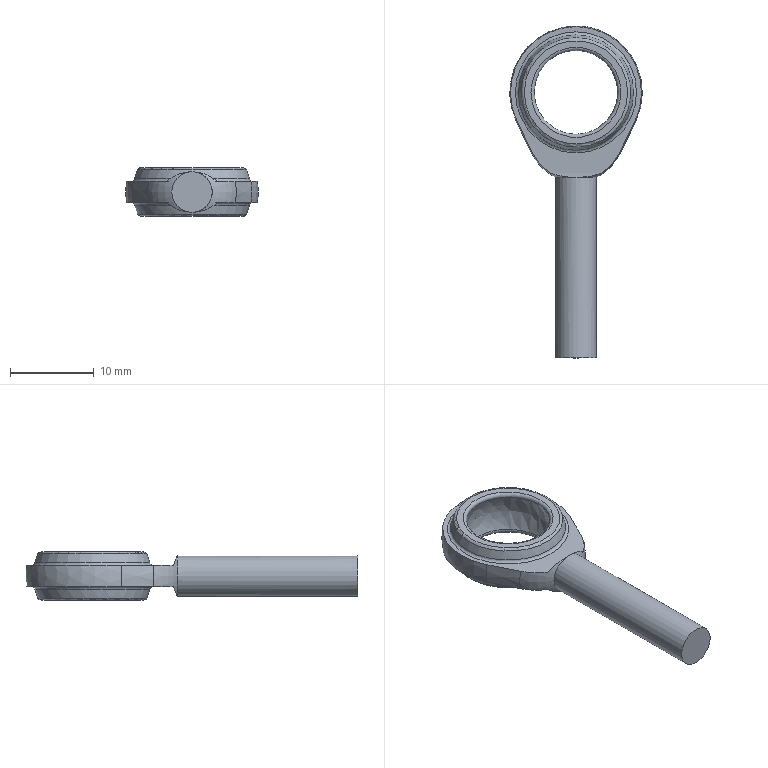Part | NX | features 59915K271(body) 2 | 1 solid | 22 faces | box 15.875 x 39.688 x 5.766 mm | volume 906.997 mm3 | torus 8 | plane 7 | sphere 4 | cone 2 | cylinder 1 | commonest cylinder face diameters 4.826 x1
STEP:
#1=CARTESIAN_POINT('',(0.,17.404,1.27));
#2=VERTEX_POINT('',#1);
#3=CARTESIAN_POINT('',(0.,10.16,1.27));
#4=DIRECTION('',(0.,0.,-1.));
#5=DIRECTION('',(0.,1.,0.));
#6=AXIS2_PLACEMENT_3D('',#3,#4,#5);
#7=CIRCLE('',#6,7.244);
#8=EDGE_CURVE('',#2,#2,#7,.T.);
#9=ORIENTED_EDGE('',*,*,#8,.T.);
#10=EDGE_LOOP('',(#9));
#11=FACE_BOUND('',#10,.T.);
#12=CARTESIAN_POINT('',(7.038,6.716,1.27));
#13=VERTEX_POINT('',#12);
#14=CARTESIAN_POINT('',(5.152,2.886,1.27));
#15=VERTEX_POINT('',#14);
#16=CARTESIAN_POINT('',(7.038,6.716,1.27));
#17=CARTESIAN_POINT('',(6.412,5.438,1.27));
#18=CARTESIAN_POINT('',(5.785,4.161,1.27));
#19=CARTESIAN_POINT('',(5.152,2.886,1.27));
#20=B_SPLINE_CURVE_WITH_KNOTS('',3,(#16,#17,#18,#19),.UNSPECIFIED.,.F.,.F.,(4,4),(0.009879,0.01415),.UNSPECIFIED.);
#21=EDGE_CURVE('',#13,#15,#20,.T.);
#22=ORIENTED_EDGE('',*,*,#21,.F.);
#23=CARTESIAN_POINT('',(-7.038,6.716,1.27));
#24=VERTEX_POINT('',#23);
#25=CARTESIAN_POINT('',(0.,10.16,1.27));
#26=DIRECTION('',(0.,0.,-1.));
#27=DIRECTION('',(0.,1.,0.));
#28=AXIS2_PLACEMENT_3D('',#25,#26,#27);
#29=CIRCLE('',#28,7.835);
#30=EDGE_CURVE('',#24,#13,#29,.T.);
#31=ORIENTED_EDGE('',*,*,#30,.F.);
#32=CARTESIAN_POINT('',(-5.152,2.886,1.27));
#33=VERTEX_POINT('',#32);
#34=CARTESIAN_POINT('',(-5.152,2.886,1.27));
#35=CARTESIAN_POINT('',(-5.785,4.161,1.27));
#36=CARTESIAN_POINT('',(-6.412,5.438,1.27));
#37=CARTESIAN_POINT('',(-7.038,6.716,1.27));
#38=B_SPLINE_CURVE_WITH_KNOTS('',3,(#34,#35,#36,#37),.UNSPECIFIED.,.F.,.F.,(4,4),(0.03405,0.03828),.UNSPECIFIED.);
#39=EDGE_CURVE('',#33,#24,#38,.T.);
#40=ORIENTED_EDGE('',*,*,#39,.F.);
#41=CARTESIAN_POINT('',(-3.029,0.508,1.27));
#42=VERTEX_POINT('',#41);
#43=CARTESIAN_POINT('',(-3.029,0.508,1.27));
#44=CARTESIAN_POINT('',(-3.94,1.095,1.27));
#45=CARTESIAN_POINT('',(-4.677,1.926,1.27));
#46=CARTESIAN_POINT('',(-5.152,2.886,1.27));
#47=B_SPLINE_CURVE_WITH_KNOTS('',3,(#43,#44,#45,#46),.UNSPECIFIED.,.F.,.F.,(4,4),(0.00321,0.006446),.UNSPECIFIED.);
#48=EDGE_CURVE('',#42,#33,#47,.T.);
#49=ORIENTED_EDGE('',*,*,#48,.F.);
#50=CARTESIAN_POINT('',(3.029,0.508,1.27));
#51=VERTEX_POINT('',#50);
#52=CARTESIAN_POINT('',(-7.938,0.508,1.27));
#53=DIRECTION('',(1.,0.,0.));
#54=VECTOR('',#53,1000.);
#55=LINE('',#52,#54);
#56=EDGE_CURVE('',#42,#51,#55,.T.);
#57=ORIENTED_EDGE('',*,*,#56,.T.);
#58=CARTESIAN_POINT('',(5.152,2.886,1.27));
#59=CARTESIAN_POINT('',(4.677,1.927,1.27));
#60=CARTESIAN_POINT('',(3.932,1.09,1.27));
#61=CARTESIAN_POINT('',(3.029,0.508,1.27));
#62=B_SPLINE_CURVE_WITH_KNOTS('',3,(#58,#59,#60,#61),.UNSPECIFIED.,.F.,.F.,(4,4),(0.03046,0.0337),.UNSPECIFIED.);
#63=EDGE_CURVE('',#15,#51,#62,.T.);
#64=ORIENTED_EDGE('',*,*,#63,.F.);
#65=EDGE_LOOP('',(#22,#31,#40,#49,#57,#64));
#66=FACE_BOUND('',#65,.T.);
#67=CARTESIAN_POINT('',(-7.938,18.098,1.27));
#68=DIRECTION('',(0.,0.,-1.));
#69=DIRECTION('',(0.,1.,0.));
#70=AXIS2_PLACEMENT_3D('',#67,#68,#69);
#71=PLANE('',#70);
#72=ADVANCED_FACE('',(#11,#66),#71,.F.);
#73=CARTESIAN_POINT('',(0.,2.916,-1.27));
#74=VERTEX_POINT('',#73);
#75=CARTESIAN_POINT('',(0.,10.16,-1.27));
#76=DIRECTION('',(0.,0.,1.));
#77=DIRECTION('',(0.,-1.,0.));
#78=AXIS2_PLACEMENT_3D('',#75,#76,#77);
#79=CIRCLE('',#78,7.244);
#80=EDGE_CURVE('',#74,#74,#79,.T.);
#81=ORIENTED_EDGE('',*,*,#80,.T.);
#82=EDGE_LOOP('',(#81));
#83=FACE_BOUND('',#82,.T.);
#84=CARTESIAN_POINT('',(-7.038,6.716,-1.27));
#85=VERTEX_POINT('',#84);
#86=CARTESIAN_POINT('',(-5.152,2.886,-1.27));
#87=VERTEX_POINT('',#86);
#88=CARTESIAN_POINT('',(-7.038,6.716,-1.27));
#89=CARTESIAN_POINT('',(-6.412,5.438,-1.27));
#90=CARTESIAN_POINT('',(-5.785,4.161,-1.27));
#91=CARTESIAN_POINT('',(-5.152,2.886,-1.27));
#92=B_SPLINE_CURVE_WITH_KNOTS('',3,(#88,#89,#90,#91),.UNSPECIFIED.,.F.,.F.,(4,4),(0.009879,0.01415),.UNSPECIFIED.);
#93=EDGE_CURVE('',#85,#87,#92,.T.);
#94=ORIENTED_EDGE('',*,*,#93,.F.);
#95=CARTESIAN_POINT('',(7.038,6.716,-1.27));
#96=VERTEX_POINT('',#95);
#97=CARTESIAN_POINT('',(0.,10.16,-1.27));
#98=DIRECTION('',(0.,0.,1.));
#99=DIRECTION('',(0.,-1.,0.));
#100=AXIS2_PLACEMENT_3D('',#97,#98,#99);
#101=CIRCLE('',#100,7.835);
#102=EDGE_CURVE('',#96,#85,#101,.T.);
#103=ORIENTED_EDGE('',*,*,#102,.F.);
#104=CARTESIAN_POINT('',(5.152,2.886,-1.27));
#105=VERTEX_POINT('',#104);
#106=CARTESIAN_POINT('',(5.152,2.886,-1.27));
#107=CARTESIAN_POINT('',(5.785,4.161,-1.27));
#108=CARTESIAN_POINT('',(6.412,5.438,-1.27));
#109=CARTESIAN_POINT('',(7.038,6.716,-1.27));
#110=B_SPLINE_CURVE_WITH_KNOTS('',3,(#106,#107,#108,#109),.UNSPECIFIED.,.F.,.F.,(4,4),(0.03405,0.03828),.UNSPECIFIED.);
#111=EDGE_CURVE('',#105,#96,#110,.T.);
#112=ORIENTED_EDGE('',*,*,#111,.F.);
#113=CARTESIAN_POINT('',(3.029,0.508,-1.27));
#114=VERTEX_POINT('',#113);
#115=CARTESIAN_POINT('',(3.029,0.508,-1.27));
#116=CARTESIAN_POINT('',(3.94,1.095,-1.27));
#117=CARTESIAN_POINT('',(4.677,1.926,-1.27));
#118=CARTESIAN_POINT('',(5.152,2.886,-1.27));
#119=B_SPLINE_CURVE_WITH_KNOTS('',3,(#115,#116,#117,#118),.UNSPECIFIED.,.F.,.F.,(4,4),(0.00321,0.006446),.UNSPECIFIED.);
#120=EDGE_CURVE('',#114,#105,#119,.T.);
#121=ORIENTED_EDGE('',*,*,#120,.F.);
#122=CARTESIAN_POINT('',(-3.029,0.508,-1.27));
#123=VERTEX_POINT('',#122);
#124=CARTESIAN_POINT('',(-7.938,0.508,-1.27));
#125=DIRECTION('',(1.,0.,0.));
#126=VECTOR('',#125,1000.);
#127=LINE('',#124,#126);
#128=EDGE_CURVE('',#123,#114,#127,.T.);
#129=ORIENTED_EDGE('',*,*,#128,.F.);
#130=CARTESIAN_POINT('',(-5.152,2.886,-1.27));
#131=CARTESIAN_POINT('',(-4.677,1.927,-1.27));
#132=CARTESIAN_POINT('',(-3.932,1.09,-1.27));
#133=CARTESIAN_POINT('',(-3.029,0.508,-1.27));
#134=B_SPLINE_CURVE_WITH_KNOTS('',3,(#130,#131,#132,#133),.UNSPECIFIED.,.F.,.F.,(4,4),(0.03046,0.0337),.UNSPECIFIED.);
#135=EDGE_CURVE('',#87,#123,#134,.T.);
#136=ORIENTED_EDGE('',*,*,#135,.F.);
#137=EDGE_LOOP('',(#94,#103,#112,#121,#129,#136));
#138=FACE_BOUND('',#137,.T.);
#139=CARTESIAN_POINT('',(-7.938,18.098,-1.27));
#140=DIRECTION('',(0.,0.,1.));
#141=DIRECTION('',(0.,-1.,0.));
#142=AXIS2_PLACEMENT_3D('',#139,#140,#141);
#143=PLANE('',#142);
#144=ADVANCED_FACE('',(#83,#138),#143,.F.);
#145=CARTESIAN_POINT('',(0.,0.,-2.413));
#146=VERTEX_POINT('',#145);
#147=CARTESIAN_POINT('',(0.,0.,-2.413));
#148=CARTESIAN_POINT('',(1.116,0.,-2.413));
#149=CARTESIAN_POINT('',(2.225,0.1858,-1.995));
#150=CARTESIAN_POINT('',(3.029,0.508,-1.27));
#151=B_SPLINE_CURVE_WITH_KNOTS('',3,(#147,#148,#149,#150),.UNSPECIFIED.,.F.,.F.,(4,4),(0.003344,0.006684),.UNSPECIFIED.);
#152=EDGE_CURVE('',#146,#114,#151,.T.);
#153=ORIENTED_EDGE('',*,*,#152,.T.);
#154=ORIENTED_EDGE('',*,*,#120,.T.);
#155=CARTESIAN_POINT('',(0.,2.886,0.));
#156=DIRECTION('',(0.,1.,0.));
#157=DIRECTION('',(-1.,0.,0.));
#158=AXIS2_PLACEMENT_3D('',#155,#156,#157);
#159=CIRCLE('',#158,5.307);
#160=EDGE_CURVE('',#15,#105,#159,.T.);
#161=ORIENTED_EDGE('',*,*,#160,.F.);
#162=ORIENTED_EDGE('',*,*,#63,.T.);
#163=CARTESIAN_POINT('',(0.,0.,2.413));
#164=VERTEX_POINT('',#163);
#165=CARTESIAN_POINT('',(3.029,0.508,1.27));
#166=CARTESIAN_POINT('',(2.224,0.1855,1.996));
#167=CARTESIAN_POINT('',(1.118,0.,2.413));
#168=CARTESIAN_POINT('',(0.,0.,2.413));
#169=B_SPLINE_CURVE_WITH_KNOTS('',3,(#165,#166,#167,#168),.UNSPECIFIED.,.F.,.F.,(4,4),(0.000000307,0.003344),.UNSPECIFIED.);
#170=EDGE_CURVE('',#51,#164,#169,.T.);
#171=ORIENTED_EDGE('',*,*,#170,.T.);
#172=CARTESIAN_POINT('',(0.,0.,0.));
#173=DIRECTION('',(0.,1.,0.));
#174=DIRECTION('',(-1.,0.,0.));
#175=AXIS2_PLACEMENT_3D('',#172,#173,#174);
#176=CIRCLE('',#175,2.413);
#177=EDGE_CURVE('',#164,#146,#176,.T.);
#178=ORIENTED_EDGE('',*,*,#177,.T.);
#179=EDGE_LOOP('',(#153,#154,#161,#162,#171,#178));
#180=FACE_BOUND('',#179,.T.);
#181=CARTESIAN_POINT('',(0.,5.56,0.));
#182=DIRECTION('',(0.,1.,0.));
#183=DIRECTION('',(-1.,0.,0.));
#184=AXIS2_PLACEMENT_3D('',#181,#182,#183);
#185=DEGENERATE_TOROIDAL_SURFACE('',#184,0.2462,6.163,.F.);
#186=ADVANCED_FACE('',(#180),#185,.F.);
#187=CARTESIAN_POINT('',(0.,6.716,0.));
#188=DIRECTION('',(0.,1.,0.));
#189=DIRECTION('',(-1.,0.,0.));
#190=AXIS2_PLACEMENT_3D('',#187,#188,#189);
#191=CIRCLE('',#190,7.151);
#192=EDGE_CURVE('',#85,#24,#191,.T.);
#193=ORIENTED_EDGE('',*,*,#192,.F.);
#194=ORIENTED_EDGE('',*,*,#93,.T.);
#195=CARTESIAN_POINT('',(0.,2.886,0.));
#196=DIRECTION('',(0.,1.,0.));
#197=DIRECTION('',(-1.,0.,0.));
#198=AXIS2_PLACEMENT_3D('',#195,#196,#197);
#199=CIRCLE('',#198,5.307);
#200=EDGE_CURVE('',#87,#33,#199,.T.);
#201=ORIENTED_EDGE('',*,*,#200,.T.);
#202=ORIENTED_EDGE('',*,*,#39,.T.);
#203=EDGE_LOOP('',(#193,#194,#201,#202));
#204=FACE_BOUND('',#203,.T.);
#205=CARTESIAN_POINT('',(0.,2.886,0.));
#206=DIRECTION('',(0.,1.,0.));
#207=DIRECTION('',(-1.,0.,0.));
#208=AXIS2_PLACEMENT_3D('',#205,#206,#207);
#209=CONICAL_SURFACE('',#208,5.307,0.4488);
#210=ADVANCED_FACE('',(#204),#209,.T.);
#211=ORIENTED_EDGE('',*,*,#177,.F.);
#212=CARTESIAN_POINT('',(0.,0.,0.));
#213=DIRECTION('',(0.,1.,0.));
#214=DIRECTION('',(-1.,0.,0.));
#215=AXIS2_PLACEMENT_3D('',#212,#213,#214);
#216=CIRCLE('',#215,2.413);
#217=EDGE_CURVE('',#146,#164,#216,.T.);
#218=ORIENTED_EDGE('',*,*,#217,.F.);
#219=EDGE_LOOP('',(#211,#218));
#220=FACE_BOUND('',#219,.T.);
#221=CARTESIAN_POINT('',(-2.413,-21.59,0.));
#222=VERTEX_POINT('',#221);
#223=CARTESIAN_POINT('',(0.,-21.59,0.));
#224=DIRECTION('',(0.,1.,0.));
#225=DIRECTION('',(-1.,0.,0.));
#226=AXIS2_PLACEMENT_3D('',#223,#224,#225);
#227=CIRCLE('',#226,2.413);
#228=EDGE_CURVE('',#222,#222,#227,.T.);
#229=ORIENTED_EDGE('',*,*,#228,.T.);
#230=EDGE_LOOP('',(#229));
#231=FACE_BOUND('',#230,.T.);
#232=CARTESIAN_POINT('',(0.,18.098,0.));
#233=DIRECTION('',(0.,1.,0.));
#234=DIRECTION('',(-1.,0.,0.));
#235=AXIS2_PLACEMENT_3D('',#232,#233,#234);
#236=CYLINDRICAL_SURFACE('',#235,2.413);
#237=ADVANCED_FACE('',(#220,#231),#236,.T.);
#238=ORIENTED_EDGE('',*,*,#228,.F.);
#239=EDGE_LOOP('',(#238));
#240=FACE_BOUND('',#239,.T.);
#241=CARTESIAN_POINT('',(0.,-21.59,0.));
#242=DIRECTION('',(0.,1.,0.));
#243=DIRECTION('',(-1.,0.,0.));
#244=AXIS2_PLACEMENT_3D('',#241,#242,#243);
#245=PLANE('',#244);
#246=ADVANCED_FACE('',(#240),#245,.F.);
#247=CARTESIAN_POINT('',(0.,6.716,0.));
#248=DIRECTION('',(0.,1.,0.));
#249=DIRECTION('',(-1.,0.,0.));
#250=AXIS2_PLACEMENT_3D('',#247,#248,#249);
#251=CIRCLE('',#250,7.151);
#252=EDGE_CURVE('',#13,#96,#251,.T.);
#253=ORIENTED_EDGE('',*,*,#252,.T.);
#254=ORIENTED_EDGE('',*,*,#102,.T.);
#255=ORIENTED_EDGE('',*,*,#192,.T.);
#256=ORIENTED_EDGE('',*,*,#30,.T.);
#257=EDGE_LOOP('',(#253,#254,#255,#256));
#258=FACE_BOUND('',#257,.T.);
#259=CARTESIAN_POINT('',(0.,10.16,0.));
#260=DIRECTION('',(0.,1.,0.));
#261=DIRECTION('',(1.,0.,0.));
#262=AXIS2_PLACEMENT_3D('',#259,#260,#261);
#263=SPHERICAL_SURFACE('',#262,7.938);
#264=ADVANCED_FACE('',(#258),#263,.T.);
#265=ORIENTED_EDGE('',*,*,#200,.F.);
#266=ORIENTED_EDGE('',*,*,#135,.T.);
#267=CARTESIAN_POINT('',(-3.029,0.508,-1.27));
#268=CARTESIAN_POINT('',(-2.224,0.1855,-1.996));
#269=CARTESIAN_POINT('',(-1.118,0.,-2.413));
#270=CARTESIAN_POINT('',(0.,0.,-2.413));
#271=B_SPLINE_CURVE_WITH_KNOTS('',3,(#267,#268,#269,#270),.UNSPECIFIED.,.F.,.F.,(4,4),(0.000000307,0.003344),.UNSPECIFIED.);
#272=EDGE_CURVE('',#123,#146,#271,.T.);
#273=ORIENTED_EDGE('',*,*,#272,.T.);
#274=ORIENTED_EDGE('',*,*,#217,.T.);
#275=CARTESIAN_POINT('',(0.,0.,2.413));
#276=CARTESIAN_POINT('',(-1.116,0.,2.413));
#277=CARTESIAN_POINT('',(-2.225,0.1858,1.995));
#278=CARTESIAN_POINT('',(-3.029,0.508,1.27));
#279=B_SPLINE_CURVE_WITH_KNOTS('',3,(#275,#276,#277,#278),.UNSPECIFIED.,.F.,.F.,(4,4),(0.003344,0.006684),.UNSPECIFIED.);
#280=EDGE_CURVE('',#164,#42,#279,.T.);
#281=ORIENTED_EDGE('',*,*,#280,.T.);
#282=ORIENTED_EDGE('',*,*,#48,.T.);
#283=EDGE_LOOP('',(#265,#266,#273,#274,#281,#282));
#284=FACE_BOUND('',#283,.T.);
#285=CARTESIAN_POINT('',(0.,5.56,0.));
#286=DIRECTION('',(0.,1.,0.));
#287=DIRECTION('',(-1.,0.,0.));
#288=AXIS2_PLACEMENT_3D('',#285,#286,#287);
#289=DEGENERATE_TOROIDAL_SURFACE('',#288,0.2462,6.163,.F.);
#290=ADVANCED_FACE('',(#284),#289,.F.);
#291=ORIENTED_EDGE('',*,*,#160,.T.);
#292=ORIENTED_EDGE('',*,*,#111,.T.);
#293=ORIENTED_EDGE('',*,*,#252,.F.);
#294=ORIENTED_EDGE('',*,*,#21,.T.);
#295=EDGE_LOOP('',(#291,#292,#293,#294));
#296=FACE_BOUND('',#295,.T.);
#297=CARTESIAN_POINT('',(0.,2.886,0.));
#298=DIRECTION('',(0.,1.,0.));
#299=DIRECTION('',(-1.,0.,0.));
#300=AXIS2_PLACEMENT_3D('',#297,#298,#299);
#301=CONICAL_SURFACE('',#300,5.307,0.4488);
#302=ADVANCED_FACE('',(#296),#301,.T.);
#303=ORIENTED_EDGE('',*,*,#56,.F.);
#304=ORIENTED_EDGE('',*,*,#280,.F.);
#305=ORIENTED_EDGE('',*,*,#170,.F.);
#306=EDGE_LOOP('',(#303,#304,#305));
#307=FACE_BOUND('',#306,.T.);
#308=CARTESIAN_POINT('',(-7.938,0.,2.413));
#309=DIRECTION('',(0.,-0.9138,-0.4061));
#310=DIRECTION('',(0.,0.4061,-0.9138));
#311=AXIS2_PLACEMENT_3D('',#308,#309,#310);
#312=PLANE('',#311);
#313=ADVANCED_FACE('',(#307),#312,.F.);
#314=ORIENTED_EDGE('',*,*,#128,.T.);
#315=ORIENTED_EDGE('',*,*,#152,.F.);
#316=ORIENTED_EDGE('',*,*,#272,.F.);
#317=EDGE_LOOP('',(#314,#315,#316));
#318=FACE_BOUND('',#317,.T.);
#319=CARTESIAN_POINT('',(-7.938,0.,-2.413));
#320=DIRECTION('',(0.,-0.9138,0.4061));
#321=DIRECTION('',(0.,-0.4061,-0.9138));
#322=AXIS2_PLACEMENT_3D('',#319,#320,#321);
#323=PLANE('',#322);
#324=ADVANCED_FACE('',(#318),#323,.F.);
#325=CARTESIAN_POINT('',(0.,3.288,-1.566));
#326=VERTEX_POINT('',#325);
#327=CARTESIAN_POINT('',(0.,10.16,-1.566));
#328=DIRECTION('',(0.,0.,1.));
#329=DIRECTION('',(0.,-1.,0.));
#330=AXIS2_PLACEMENT_3D('',#327,#328,#329);
#331=CIRCLE('',#330,6.872);
#332=EDGE_CURVE('',#326,#326,#331,.F.);
#333=ORIENTED_EDGE('',*,*,#332,.T.);
#334=EDGE_LOOP('',(#333));
#335=FACE_BOUND('',#334,.T.);
#336=CARTESIAN_POINT('',(6.533,10.16,-2.645));
#337=VERTEX_POINT('',#336);
#338=CARTESIAN_POINT('',(0.,10.16,-2.645));
#339=DIRECTION('',(0.,0.,1.));
#340=DIRECTION('',(1.,0.,0.));
#341=AXIS2_PLACEMENT_3D('',#338,#339,#340);
#342=CIRCLE('',#341,6.533);
#343=EDGE_CURVE('',#337,#337,#342,.T.);
#344=ORIENTED_EDGE('',*,*,#343,.T.);
#345=EDGE_LOOP('',(#344));
#346=FACE_BOUND('',#345,.T.);
#347=CARTESIAN_POINT('',(0.,10.16,0.));
#348=DIRECTION('',(0.,0.,1.));
#349=DIRECTION('',(0.,1.,0.));
#350=AXIS2_PLACEMENT_3D('',#347,#348,#349);
#351=SPHERICAL_SURFACE('',#350,7.048);
#352=ADVANCED_FACE('',(#335,#346),#351,.T.);
#353=CARTESIAN_POINT('',(5.377,10.16,-2.883));
#354=VERTEX_POINT('',#353);
#355=CARTESIAN_POINT('',(0.,10.16,-2.883));
#356=DIRECTION('',(0.,0.,1.));
#357=DIRECTION('',(1.,0.,0.));
#358=AXIS2_PLACEMENT_3D('',#355,#356,#357);
#359=CIRCLE('',#358,5.377);
#360=EDGE_CURVE('',#354,#354,#359,.T.);
#361=ORIENTED_EDGE('',*,*,#360,.T.);
#362=EDGE_LOOP('',(#361));
#363=FACE_BOUND('',#362,.T.);
#364=CARTESIAN_POINT('',(6.18,10.16,-2.883));
#365=VERTEX_POINT('',#364);
#366=CARTESIAN_POINT('',(0.,10.16,-2.883));
#367=DIRECTION('',(0.,0.,1.));
#368=DIRECTION('',(1.,0.,0.));
#369=AXIS2_PLACEMENT_3D('',#366,#367,#368);
#370=CIRCLE('',#369,6.18);
#371=EDGE_CURVE('',#365,#365,#370,.F.);
#372=ORIENTED_EDGE('',*,*,#371,.T.);
#373=EDGE_LOOP('',(#372));
#374=FACE_BOUND('',#373,.T.);
#375=CARTESIAN_POINT('',(0.,16.592,-2.883));
#376=DIRECTION('',(0.,0.,1.));
#377=DIRECTION('',(1.,0.,0.));
#378=AXIS2_PLACEMENT_3D('',#375,#376,#377);
#379=PLANE('',#378);
#380=ADVANCED_FACE('',(#363,#374),#379,.F.);
#381=CARTESIAN_POINT('',(0.,17.032,1.566));
#382=VERTEX_POINT('',#381);
#383=CARTESIAN_POINT('',(0.,10.16,1.566));
#384=DIRECTION('',(0.,0.,-1.));
#385=DIRECTION('',(0.,1.,0.));
#386=AXIS2_PLACEMENT_3D('',#383,#384,#385);
#387=CIRCLE('',#386,6.872);
#388=EDGE_CURVE('',#382,#382,#387,.F.);
#389=ORIENTED_EDGE('',*,*,#388,.T.);
#390=EDGE_LOOP('',(#389));
#391=FACE_BOUND('',#390,.T.);
#392=CARTESIAN_POINT('',(-6.533,10.16,2.645));
#393=VERTEX_POINT('',#392);
#394=CARTESIAN_POINT('',(0.,10.16,2.645));
#395=DIRECTION('',(0.,0.,-1.));
#396=DIRECTION('',(-1.,0.,0.));
#397=AXIS2_PLACEMENT_3D('',#394,#395,#396);
#398=CIRCLE('',#397,6.533);
#399=EDGE_CURVE('',#393,#393,#398,.T.);
#400=ORIENTED_EDGE('',*,*,#399,.T.);
#401=EDGE_LOOP('',(#400));
#402=FACE_BOUND('',#401,.T.);
#403=CARTESIAN_POINT('',(0.,10.16,0.));
#404=DIRECTION('',(0.,0.,1.));
#405=DIRECTION('',(0.,1.,0.));
#406=AXIS2_PLACEMENT_3D('',#403,#404,#405);
#407=SPHERICAL_SURFACE('',#406,7.048);
#408=ADVANCED_FACE('',(#391,#402),#407,.T.);
#409=CARTESIAN_POINT('',(-5.377,10.16,2.883));
#410=VERTEX_POINT('',#409);
#411=CARTESIAN_POINT('',(0.,10.16,2.883));
#412=DIRECTION('',(0.,0.,-1.));
#413=DIRECTION('',(-1.,0.,0.));
#414=AXIS2_PLACEMENT_3D('',#411,#412,#413);
#415=CIRCLE('',#414,5.377);
#416=EDGE_CURVE('',#410,#410,#415,.T.);
#417=ORIENTED_EDGE('',*,*,#416,.T.);
#418=EDGE_LOOP('',(#417));
#419=FACE_BOUND('',#418,.T.);
#420=CARTESIAN_POINT('',(-6.18,10.16,2.883));
#421=VERTEX_POINT('',#420);
#422=CARTESIAN_POINT('',(0.,10.16,2.883));
#423=DIRECTION('',(0.,0.,-1.));
#424=DIRECTION('',(-1.,0.,0.));
#425=AXIS2_PLACEMENT_3D('',#422,#423,#424);
#426=CIRCLE('',#425,6.18);
#427=EDGE_CURVE('',#421,#421,#426,.F.);
#428=ORIENTED_EDGE('',*,*,#427,.T.);
#429=EDGE_LOOP('',(#428));
#430=FACE_BOUND('',#429,.T.);
#431=CARTESIAN_POINT('',(0.,16.592,2.883));
#432=DIRECTION('',(0.,0.,-1.));
#433=DIRECTION('',(-1.,0.,0.));
#434=AXIS2_PLACEMENT_3D('',#431,#432,#433);
#435=PLANE('',#434);
#436=ADVANCED_FACE('',(#419,#430),#435,.F.);
#437=CARTESIAN_POINT('',(5.032,10.16,-2.341));
#438=VERTEX_POINT('',#437);
#439=CARTESIAN_POINT('',(0.,10.16,-2.341));
#440=DIRECTION('',(0.,0.,1.));
#441=DIRECTION('',(1.,0.,0.));
#442=AXIS2_PLACEMENT_3D('',#439,#440,#441);
#443=CIRCLE('',#442,5.032);
#444=EDGE_CURVE('',#438,#438,#443,.F.);
#445=ORIENTED_EDGE('',*,*,#444,.T.);
#446=EDGE_LOOP('',(#445));
#447=FACE_BOUND('',#446,.T.);
#448=CARTESIAN_POINT('',(-5.032,10.16,2.341));
#449=VERTEX_POINT('',#448);
#450=CARTESIAN_POINT('',(0.,10.16,2.341));
#451=DIRECTION('',(0.,0.,-1.));
#452=DIRECTION('',(-1.,0.,0.));
#453=AXIS2_PLACEMENT_3D('',#450,#451,#452);
#454=CIRCLE('',#453,5.032);
#455=EDGE_CURVE('',#449,#449,#454,.F.);
#456=ORIENTED_EDGE('',*,*,#455,.T.);
#457=EDGE_LOOP('',(#456));
#458=FACE_BOUND('',#457,.T.);
#459=CARTESIAN_POINT('',(0.,10.16,0.));
#460=DIRECTION('',(0.,1.,0.));
#461=DIRECTION('',(-1.,0.,0.));
#462=AXIS2_PLACEMENT_3D('',#459,#460,#461);
#463=SPHERICAL_SURFACE('',#462,5.55);
#464=ADVANCED_FACE('',(#447,#458),#463,.F.);
#465=ORIENTED_EDGE('',*,*,#8,.F.);
#466=EDGE_LOOP('',(#465));
#467=FACE_BOUND('',#466,.T.);
#468=ORIENTED_EDGE('',*,*,#388,.F.);
#469=EDGE_LOOP('',(#468));
#470=FACE_BOUND('',#469,.T.);
#471=CARTESIAN_POINT('',(0.,10.16,1.651));
#472=DIRECTION('',(0.,0.,-1.));
#473=DIRECTION('',(0.,1.,0.));
#474=AXIS2_PLACEMENT_3D('',#471,#472,#473);
#475=TOROIDAL_SURFACE('',#474,7.244,0.381);
#476=ADVANCED_FACE('',(#467,#470),#475,.F.);
#477=ORIENTED_EDGE('',*,*,#80,.F.);
#478=EDGE_LOOP('',(#477));
#479=FACE_BOUND('',#478,.T.);
#480=ORIENTED_EDGE('',*,*,#332,.F.);
#481=EDGE_LOOP('',(#480));
#482=FACE_BOUND('',#481,.T.);
#483=CARTESIAN_POINT('',(0.,10.16,-1.651));
#484=DIRECTION('',(0.,0.,1.));
#485=DIRECTION('',(0.,-1.,0.));
#486=AXIS2_PLACEMENT_3D('',#483,#484,#485);
#487=TOROIDAL_SURFACE('',#486,7.244,0.381);
#488=ADVANCED_FACE('',(#479,#482),#487,.F.);
#489=ORIENTED_EDGE('',*,*,#444,.F.);
#490=EDGE_LOOP('',(#489));
#491=FACE_BOUND('',#490,.T.);
#492=ORIENTED_EDGE('',*,*,#360,.F.);
#493=EDGE_LOOP('',(#492));
#494=FACE_BOUND('',#493,.T.);
#495=CARTESIAN_POINT('',(0.,10.16,-2.502));
#496=DIRECTION('',(0.,0.,1.));
#497=DIRECTION('',(1.,0.,0.));
#498=AXIS2_PLACEMENT_3D('',#495,#496,#497);
#499=TOROIDAL_SURFACE('',#498,5.377,0.381);
#500=ADVANCED_FACE('',(#491,#494),#499,.T.);
#501=ORIENTED_EDGE('',*,*,#371,.F.);
#502=EDGE_LOOP('',(#501));
#503=FACE_BOUND('',#502,.T.);
#504=ORIENTED_EDGE('',*,*,#343,.F.);
#505=EDGE_LOOP('',(#504));
#506=FACE_BOUND('',#505,.T.);
#507=CARTESIAN_POINT('',(0.,10.16,-2.502));
#508=DIRECTION('',(0.,0.,1.));
#509=DIRECTION('',(1.,0.,0.));
#510=AXIS2_PLACEMENT_3D('',#507,#508,#509);
#511=TOROIDAL_SURFACE('',#510,6.18,0.381);
#512=ADVANCED_FACE('',(#503,#506),#511,.T.);
#513=ORIENTED_EDGE('',*,*,#416,.F.);
#514=EDGE_LOOP('',(#513));
#515=FACE_BOUND('',#514,.T.);
#516=ORIENTED_EDGE('',*,*,#455,.F.);
#517=EDGE_LOOP('',(#516));
#518=FACE_BOUND('',#517,.T.);
#519=CARTESIAN_POINT('',(0.,10.16,2.502));
#520=DIRECTION('',(0.,0.,-1.));
#521=DIRECTION('',(-1.,0.,0.));
#522=AXIS2_PLACEMENT_3D('',#519,#520,#521);
#523=TOROIDAL_SURFACE('',#522,5.377,0.381);
#524=ADVANCED_FACE('',(#515,#518),#523,.T.);
#525=ORIENTED_EDGE('',*,*,#399,.F.);
#526=EDGE_LOOP('',(#525));
#527=FACE_BOUND('',#526,.T.);
#528=ORIENTED_EDGE('',*,*,#427,.F.);
#529=EDGE_LOOP('',(#528));
#530=FACE_BOUND('',#529,.T.);
#531=CARTESIAN_POINT('',(0.,10.16,2.502));
#532=DIRECTION('',(0.,0.,-1.));
#533=DIRECTION('',(-1.,0.,0.));
#534=AXIS2_PLACEMENT_3D('',#531,#532,#533);
#535=TOROIDAL_SURFACE('',#534,6.18,0.381);
#536=ADVANCED_FACE('',(#527,#530),#535,.T.);
#537=CLOSED_SHELL('',(#72,#144,#186,#210,#237,#246,#264,#290,#302,#313,#324,#352,#380,#408,#436,#464,#476,#488,#500,#512,#524,#536));
#538=MANIFOLD_SOLID_BREP('',#537);
#539=(LENGTH_UNIT()NAMED_UNIT(*)SI_UNIT(.MILLI.,.METRE.));
#540=UNCERTAINTY_MEASURE_WITH_UNIT(LENGTH_MEASURE(0.0508),#539,'','');
#541=(NAMED_UNIT(*)PLANE_ANGLE_UNIT()SI_UNIT($,.RADIAN.));
#542=(NAMED_UNIT(*)SI_UNIT($,.STERADIAN.)SOLID_ANGLE_UNIT());
#543=(GEOMETRIC_REPRESENTATION_CONTEXT(3)GLOBAL_UNCERTAINTY_ASSIGNED_CONTEXT((#540))GLOBAL_UNIT_ASSIGNED_CONTEXT((#539,#541,#542))REPRESENTATION_CONTEXT('',''));
#544=ADVANCED_BREP_SHAPE_REPRESENTATION('',(#538),#543);